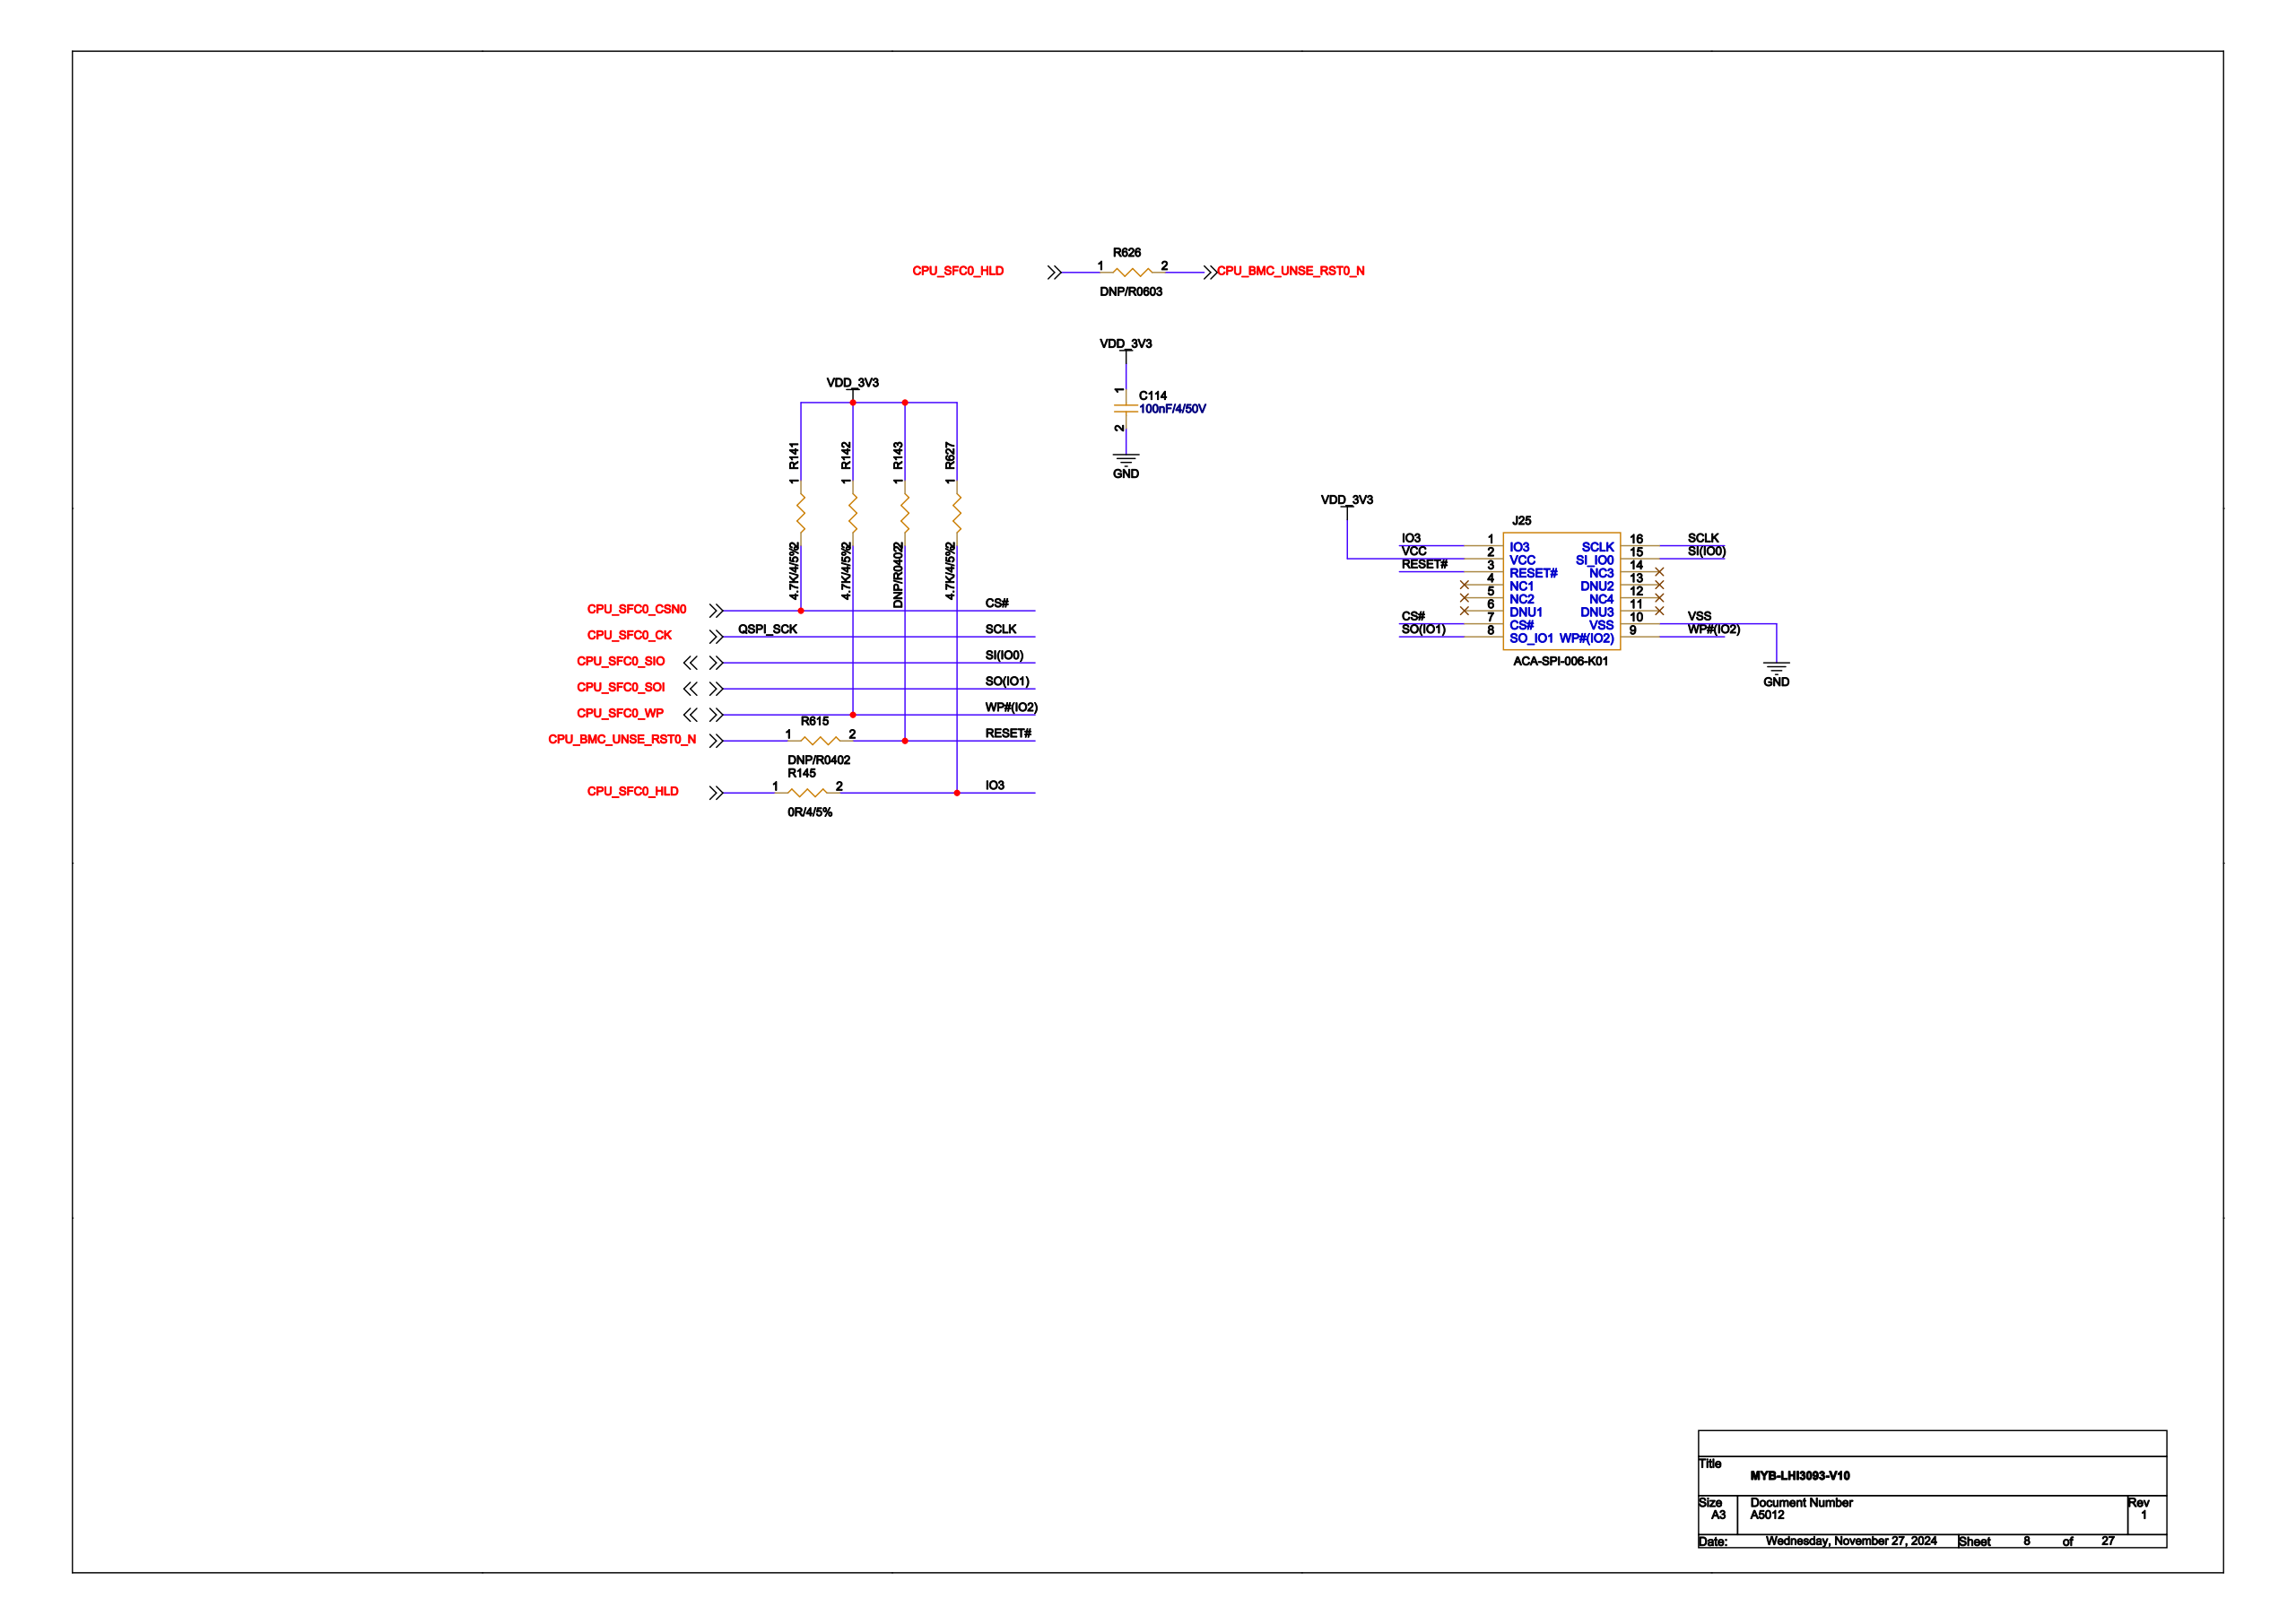Circuit board | Cadence Allegro | 1159 parts | 708 nets | one sheet of the schematic
Parts on this sheet (reference | value | footprint):
C114 | 100nF/4/50V | C0402
J25 | ACA-SPI-006-K01 | ACA-SPI-006-K01
R141 | 4.7K/4/5% | R0402
R142 | 4.7K/4/5% | R0402
R143 | DNP/R0402 | R0402
R145 | 0R/4/5% | R0402
R615 | DNP/R0402 | R0402
R626 | DNP/R0603 | R0603
R627 | 4.7K/4/5% | R0402
Nets of these parts (net: part-pin ...):
GND: C114-2 J25-10
VDD_3V3: C114-1 J25-2 R141-1 R142-1 R143-1 R627-1
CPU_SFC0_CSN0: J25-7 R141-2
IO3: J25-1 R145-2 R627-2
RESET#: J25-3 R143-2 R615-2
CPU_SFC0_CK: J25-16
CPU_SFC0_SIO: J25-15
CPU_SFC0_SOI: J25-8
CPU_SFC0_WP: J25-9 R142-2
CPU_SFC0_HLD: R145-1 R626-1
CPU_BMC_UNSE_RST0_N: R615-1 R626-2